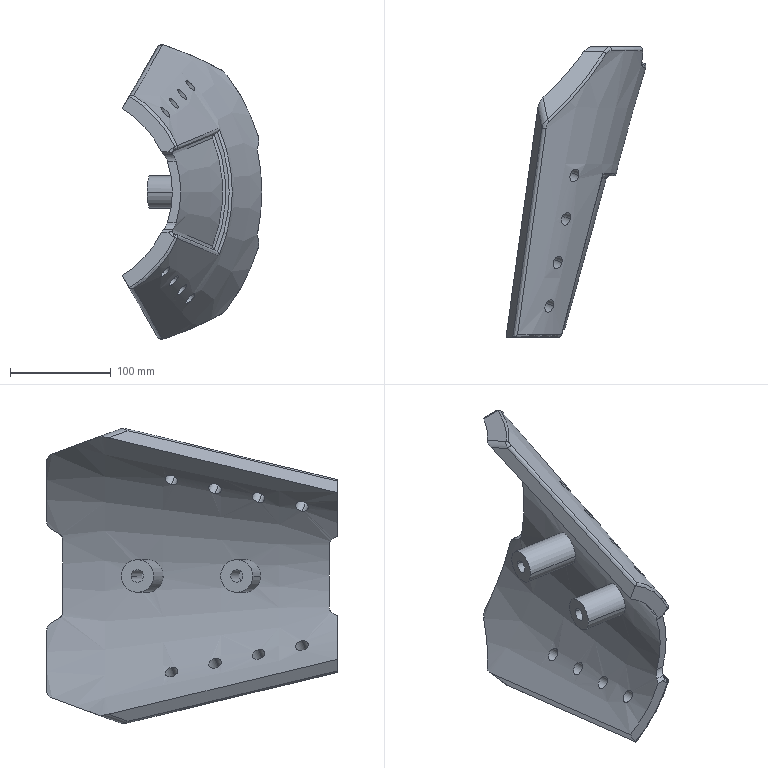Part | SolidWorks | features MirrorStock 1 | 1 solid | 91 faces | box 138.848 x 288 x 292.377 mm | volume 1252657 mm3 | cylinder 36 | spline 22 | plane 20 | torus 7 | cone 4 | sphere 2 | commonest cylinder face diameters 12.8 x16 16 x10 12.5 x4 32.5 x4 6.4 x2